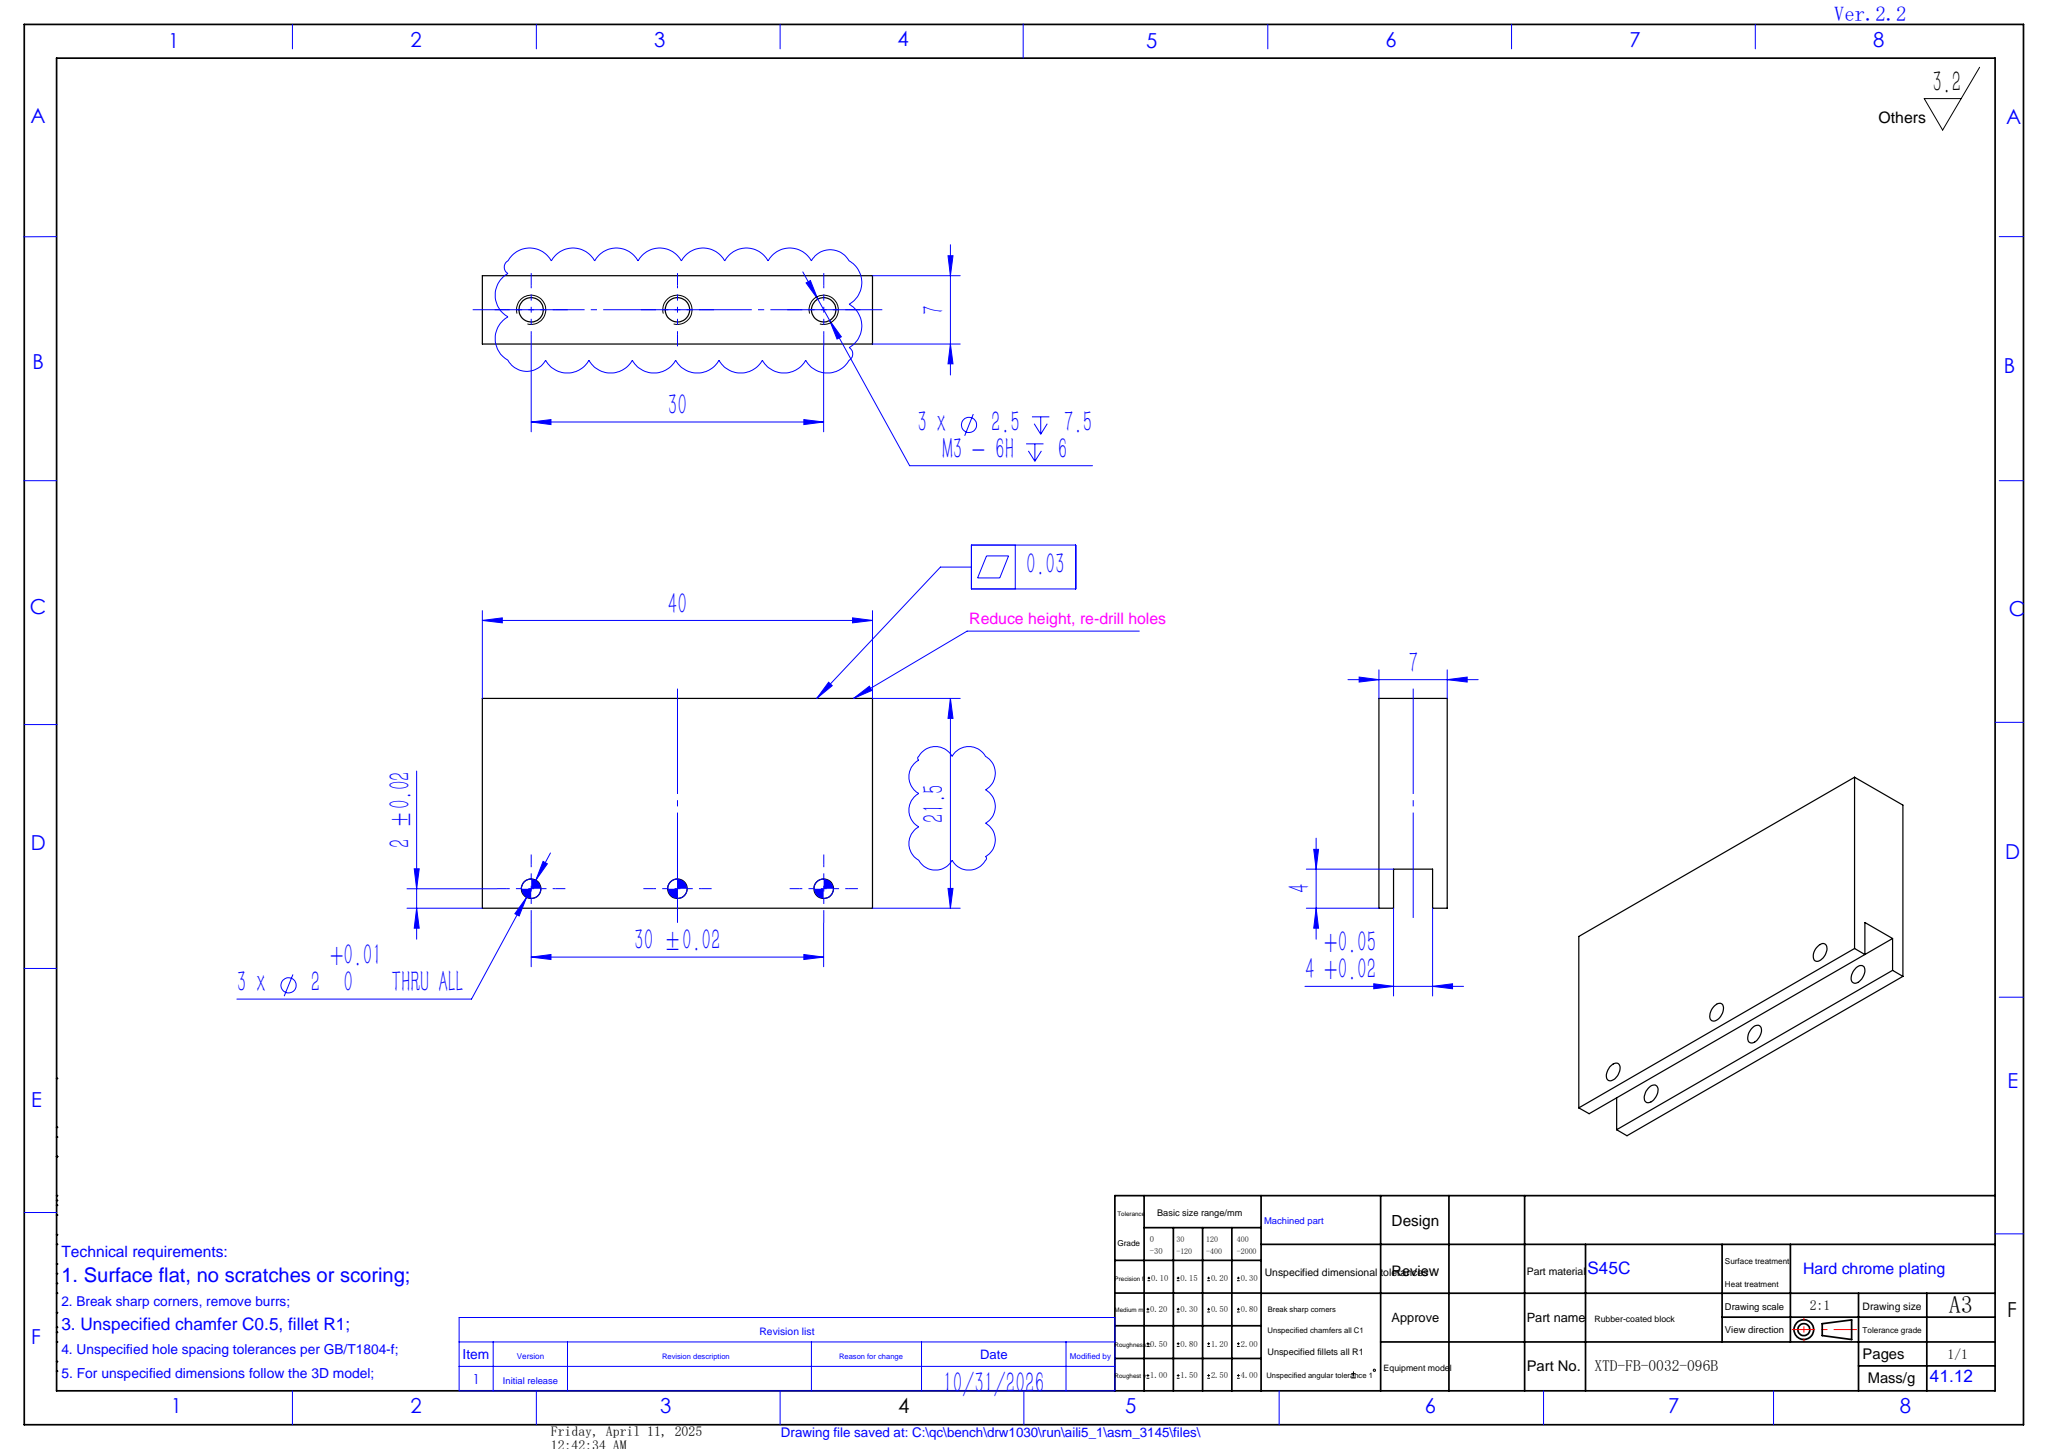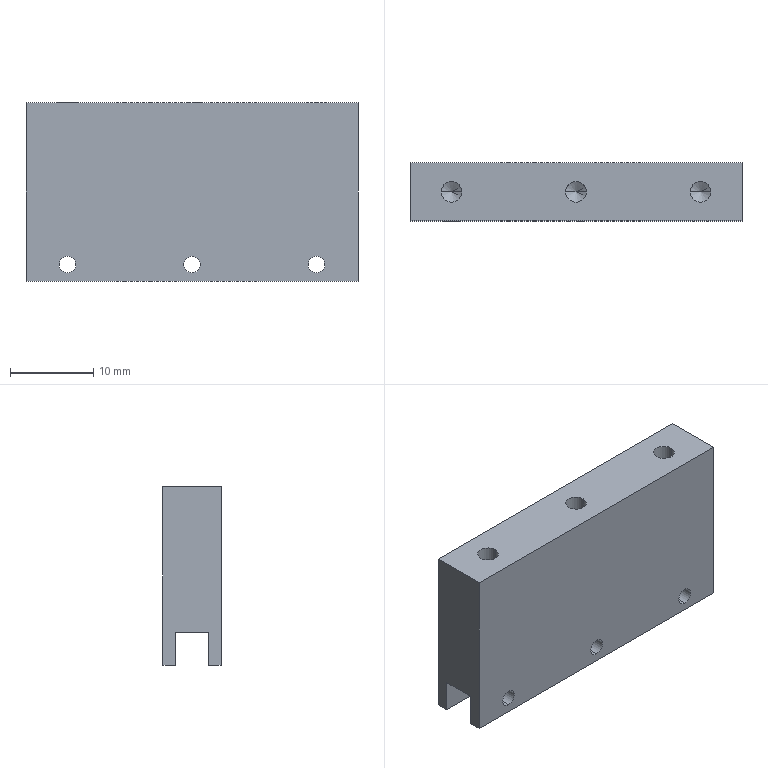Part | SolidWorks | features HoleWzd 2, Cut 1, Extrusion 1 | 1 solid | 34 faces | box 40 x 7 x 21.5 mm | volume 5238 mm3 | cylinder 18 | plane 10 | cone 6 | commonest cylinder face diameters 2 x12 2.5 x6
STEP:
#1=CARTESIAN_POINT('',(-15.,2.,1.));
#2=VERTEX_POINT('',#1);
#3=CARTESIAN_POINT('',(-15.,2.,3.));
#4=VERTEX_POINT('',#3);
#5=CARTESIAN_POINT('',(-15.,2.,2.));
#6=DIRECTION('',(0.,1.,0.));
#7=DIRECTION('',(0.,0.,1.));
#8=AXIS2_PLACEMENT_3D('',#5,#6,#7);
#9=CIRCLE('',#8,1.);
#10=EDGE_CURVE('',#2,#4,#9,.T.);
#11=ORIENTED_EDGE('',*,*,#10,.F.);
#12=CARTESIAN_POINT('',(-15.,3.5,1.));
#13=VERTEX_POINT('',#12);
#14=CARTESIAN_POINT('',(-15.,3.5,1.));
#15=DIRECTION('',(0.,1.,0.));
#16=VECTOR('',#15,1000.);
#17=LINE('',#14,#16);
#18=EDGE_CURVE('',#2,#13,#17,.T.);
#19=ORIENTED_EDGE('',*,*,#18,.T.);
#20=CARTESIAN_POINT('',(-15.,3.5,3.));
#21=VERTEX_POINT('',#20);
#22=CARTESIAN_POINT('',(-15.,3.5,2.));
#23=DIRECTION('',(0.,1.,0.));
#24=DIRECTION('',(0.,0.,1.));
#25=AXIS2_PLACEMENT_3D('',#22,#23,#24);
#26=CIRCLE('',#25,1.);
#27=EDGE_CURVE('',#13,#21,#26,.T.);
#28=ORIENTED_EDGE('',*,*,#27,.T.);
#29=CARTESIAN_POINT('',(-15.,3.5,3.));
#30=DIRECTION('',(0.,1.,0.));
#31=VECTOR('',#30,1000.);
#32=LINE('',#29,#31);
#33=EDGE_CURVE('',#4,#21,#32,.T.);
#34=ORIENTED_EDGE('',*,*,#33,.F.);
#35=EDGE_LOOP('',(#11,#19,#28,#34));
#36=FACE_OUTER_BOUND('',#35,.T.);
#37=CARTESIAN_POINT('',(-15.,3.5,2.));
#38=DIRECTION('',(0.,1.,0.));
#39=DIRECTION('',(0.,0.,1.));
#40=AXIS2_PLACEMENT_3D('',#37,#38,#39);
#41=CYLINDRICAL_SURFACE('',#40,1.);
#42=ADVANCED_FACE('',(#36),#41,.F.);
#43=CARTESIAN_POINT('',(-15.,-3.5,1.));
#44=VERTEX_POINT('',#43);
#45=CARTESIAN_POINT('',(-15.,-3.5,3.));
#46=VERTEX_POINT('',#45);
#47=CARTESIAN_POINT('',(-15.,-3.5,2.));
#48=DIRECTION('',(0.,1.,0.));
#49=DIRECTION('',(0.,0.,1.));
#50=AXIS2_PLACEMENT_3D('',#47,#48,#49);
#51=CIRCLE('',#50,1.);
#52=EDGE_CURVE('',#44,#46,#51,.T.);
#53=ORIENTED_EDGE('',*,*,#52,.F.);
#54=CARTESIAN_POINT('',(-15.,-2.,1.));
#55=VERTEX_POINT('',#54);
#56=CARTESIAN_POINT('',(-15.,3.5,1.));
#57=DIRECTION('',(0.,1.,0.));
#58=VECTOR('',#57,1000.);
#59=LINE('',#56,#58);
#60=EDGE_CURVE('',#44,#55,#59,.T.);
#61=ORIENTED_EDGE('',*,*,#60,.T.);
#62=CARTESIAN_POINT('',(-15.,-2.,3.));
#63=VERTEX_POINT('',#62);
#64=CARTESIAN_POINT('',(-15.,-2.,2.));
#65=DIRECTION('',(0.,-1.,0.));
#66=DIRECTION('',(0.,0.,-1.));
#67=AXIS2_PLACEMENT_3D('',#64,#65,#66);
#68=CIRCLE('',#67,1.);
#69=EDGE_CURVE('',#63,#55,#68,.T.);
#70=ORIENTED_EDGE('',*,*,#69,.F.);
#71=CARTESIAN_POINT('',(-15.,3.5,3.));
#72=DIRECTION('',(0.,1.,0.));
#73=VECTOR('',#72,1000.);
#74=LINE('',#71,#73);
#75=EDGE_CURVE('',#46,#63,#74,.T.);
#76=ORIENTED_EDGE('',*,*,#75,.F.);
#77=EDGE_LOOP('',(#53,#61,#70,#76));
#78=FACE_OUTER_BOUND('',#77,.T.);
#79=CARTESIAN_POINT('',(-15.,3.5,2.));
#80=DIRECTION('',(0.,1.,0.));
#81=DIRECTION('',(0.,0.,1.));
#82=AXIS2_PLACEMENT_3D('',#79,#80,#81);
#83=CYLINDRICAL_SURFACE('',#82,1.);
#84=ADVANCED_FACE('',(#78),#83,.F.);
#85=CARTESIAN_POINT('',(0.,2.,1.));
#86=VERTEX_POINT('',#85);
#87=CARTESIAN_POINT('',(0.,2.,3.));
#88=VERTEX_POINT('',#87);
#89=CARTESIAN_POINT('',(0.,2.,2.));
#90=DIRECTION('',(0.,1.,0.));
#91=DIRECTION('',(0.,0.,1.));
#92=AXIS2_PLACEMENT_3D('',#89,#90,#91);
#93=CIRCLE('',#92,1.);
#94=EDGE_CURVE('',#86,#88,#93,.T.);
#95=ORIENTED_EDGE('',*,*,#94,.F.);
#96=CARTESIAN_POINT('',(0.,3.5,1.));
#97=VERTEX_POINT('',#96);
#98=CARTESIAN_POINT('',(0.,3.5,1.));
#99=DIRECTION('',(0.,1.,0.));
#100=VECTOR('',#99,1000.);
#101=LINE('',#98,#100);
#102=EDGE_CURVE('',#86,#97,#101,.T.);
#103=ORIENTED_EDGE('',*,*,#102,.T.);
#104=CARTESIAN_POINT('',(0.,3.5,3.));
#105=VERTEX_POINT('',#104);
#106=CARTESIAN_POINT('',(0.,3.5,2.));
#107=DIRECTION('',(0.,1.,0.));
#108=DIRECTION('',(0.,0.,1.));
#109=AXIS2_PLACEMENT_3D('',#106,#107,#108);
#110=CIRCLE('',#109,1.);
#111=EDGE_CURVE('',#97,#105,#110,.T.);
#112=ORIENTED_EDGE('',*,*,#111,.T.);
#113=CARTESIAN_POINT('',(0.,3.5,3.));
#114=DIRECTION('',(0.,1.,0.));
#115=VECTOR('',#114,1000.);
#116=LINE('',#113,#115);
#117=EDGE_CURVE('',#88,#105,#116,.T.);
#118=ORIENTED_EDGE('',*,*,#117,.F.);
#119=EDGE_LOOP('',(#95,#103,#112,#118));
#120=FACE_OUTER_BOUND('',#119,.T.);
#121=CARTESIAN_POINT('',(0.,3.5,2.));
#122=DIRECTION('',(0.,1.,0.));
#123=DIRECTION('',(0.,0.,1.));
#124=AXIS2_PLACEMENT_3D('',#121,#122,#123);
#125=CYLINDRICAL_SURFACE('',#124,1.);
#126=ADVANCED_FACE('',(#120),#125,.F.);
#127=CARTESIAN_POINT('',(0.,-3.5,1.));
#128=VERTEX_POINT('',#127);
#129=CARTESIAN_POINT('',(0.,-3.5,3.));
#130=VERTEX_POINT('',#129);
#131=CARTESIAN_POINT('',(0.,-3.5,2.));
#132=DIRECTION('',(0.,1.,0.));
#133=DIRECTION('',(0.,0.,1.));
#134=AXIS2_PLACEMENT_3D('',#131,#132,#133);
#135=CIRCLE('',#134,1.);
#136=EDGE_CURVE('',#128,#130,#135,.T.);
#137=ORIENTED_EDGE('',*,*,#136,.F.);
#138=CARTESIAN_POINT('',(0.,-2.,1.));
#139=VERTEX_POINT('',#138);
#140=CARTESIAN_POINT('',(0.,3.5,1.));
#141=DIRECTION('',(0.,1.,0.));
#142=VECTOR('',#141,1000.);
#143=LINE('',#140,#142);
#144=EDGE_CURVE('',#128,#139,#143,.T.);
#145=ORIENTED_EDGE('',*,*,#144,.T.);
#146=CARTESIAN_POINT('',(0.,-2.,3.));
#147=VERTEX_POINT('',#146);
#148=CARTESIAN_POINT('',(0.,-2.,2.));
#149=DIRECTION('',(0.,-1.,0.));
#150=DIRECTION('',(0.,0.,-1.));
#151=AXIS2_PLACEMENT_3D('',#148,#149,#150);
#152=CIRCLE('',#151,1.);
#153=EDGE_CURVE('',#147,#139,#152,.T.);
#154=ORIENTED_EDGE('',*,*,#153,.F.);
#155=CARTESIAN_POINT('',(0.,3.5,3.));
#156=DIRECTION('',(0.,1.,0.));
#157=VECTOR('',#156,1000.);
#158=LINE('',#155,#157);
#159=EDGE_CURVE('',#130,#147,#158,.T.);
#160=ORIENTED_EDGE('',*,*,#159,.F.);
#161=EDGE_LOOP('',(#137,#145,#154,#160));
#162=FACE_OUTER_BOUND('',#161,.T.);
#163=CARTESIAN_POINT('',(0.,3.5,2.));
#164=DIRECTION('',(0.,1.,0.));
#165=DIRECTION('',(0.,0.,1.));
#166=AXIS2_PLACEMENT_3D('',#163,#164,#165);
#167=CYLINDRICAL_SURFACE('',#166,1.);
#168=ADVANCED_FACE('',(#162),#167,.F.);
#169=CARTESIAN_POINT('',(15.,2.,1.));
#170=VERTEX_POINT('',#169);
#171=CARTESIAN_POINT('',(15.,2.,3.));
#172=VERTEX_POINT('',#171);
#173=CARTESIAN_POINT('',(15.,2.,2.));
#174=DIRECTION('',(0.,1.,0.));
#175=DIRECTION('',(0.,0.,1.));
#176=AXIS2_PLACEMENT_3D('',#173,#174,#175);
#177=CIRCLE('',#176,1.);
#178=EDGE_CURVE('',#170,#172,#177,.T.);
#179=ORIENTED_EDGE('',*,*,#178,.F.);
#180=CARTESIAN_POINT('',(15.,3.5,1.));
#181=VERTEX_POINT('',#180);
#182=CARTESIAN_POINT('',(15.,3.5,1.));
#183=DIRECTION('',(0.,1.,0.));
#184=VECTOR('',#183,1000.);
#185=LINE('',#182,#184);
#186=EDGE_CURVE('',#170,#181,#185,.T.);
#187=ORIENTED_EDGE('',*,*,#186,.T.);
#188=CARTESIAN_POINT('',(15.,3.5,3.));
#189=VERTEX_POINT('',#188);
#190=CARTESIAN_POINT('',(15.,3.5,2.));
#191=DIRECTION('',(0.,1.,0.));
#192=DIRECTION('',(0.,0.,1.));
#193=AXIS2_PLACEMENT_3D('',#190,#191,#192);
#194=CIRCLE('',#193,1.);
#195=EDGE_CURVE('',#181,#189,#194,.T.);
#196=ORIENTED_EDGE('',*,*,#195,.T.);
#197=CARTESIAN_POINT('',(15.,3.5,3.));
#198=DIRECTION('',(0.,1.,0.));
#199=VECTOR('',#198,1000.);
#200=LINE('',#197,#199);
#201=EDGE_CURVE('',#172,#189,#200,.T.);
#202=ORIENTED_EDGE('',*,*,#201,.F.);
#203=EDGE_LOOP('',(#179,#187,#196,#202));
#204=FACE_OUTER_BOUND('',#203,.T.);
#205=CARTESIAN_POINT('',(15.,3.5,2.));
#206=DIRECTION('',(0.,1.,0.));
#207=DIRECTION('',(0.,0.,1.));
#208=AXIS2_PLACEMENT_3D('',#205,#206,#207);
#209=CYLINDRICAL_SURFACE('',#208,1.);
#210=ADVANCED_FACE('',(#204),#209,.F.);
#211=CARTESIAN_POINT('',(15.,-3.5,1.));
#212=VERTEX_POINT('',#211);
#213=CARTESIAN_POINT('',(15.,-3.5,3.));
#214=VERTEX_POINT('',#213);
#215=CARTESIAN_POINT('',(15.,-3.5,2.));
#216=DIRECTION('',(0.,1.,0.));
#217=DIRECTION('',(0.,0.,1.));
#218=AXIS2_PLACEMENT_3D('',#215,#216,#217);
#219=CIRCLE('',#218,1.);
#220=EDGE_CURVE('',#212,#214,#219,.T.);
#221=ORIENTED_EDGE('',*,*,#220,.F.);
#222=CARTESIAN_POINT('',(15.,-2.,1.));
#223=VERTEX_POINT('',#222);
#224=CARTESIAN_POINT('',(15.,3.5,1.));
#225=DIRECTION('',(0.,1.,0.));
#226=VECTOR('',#225,1000.);
#227=LINE('',#224,#226);
#228=EDGE_CURVE('',#212,#223,#227,.T.);
#229=ORIENTED_EDGE('',*,*,#228,.T.);
#230=CARTESIAN_POINT('',(15.,-2.,3.));
#231=VERTEX_POINT('',#230);
#232=CARTESIAN_POINT('',(15.,-2.,2.));
#233=DIRECTION('',(0.,-1.,0.));
#234=DIRECTION('',(0.,0.,-1.));
#235=AXIS2_PLACEMENT_3D('',#232,#233,#234);
#236=CIRCLE('',#235,1.);
#237=EDGE_CURVE('',#231,#223,#236,.T.);
#238=ORIENTED_EDGE('',*,*,#237,.F.);
#239=CARTESIAN_POINT('',(15.,3.5,3.));
#240=DIRECTION('',(0.,1.,0.));
#241=VECTOR('',#240,1000.);
#242=LINE('',#239,#241);
#243=EDGE_CURVE('',#214,#231,#242,.T.);
#244=ORIENTED_EDGE('',*,*,#243,.F.);
#245=EDGE_LOOP('',(#221,#229,#238,#244));
#246=FACE_OUTER_BOUND('',#245,.T.);
#247=CARTESIAN_POINT('',(15.,3.5,2.));
#248=DIRECTION('',(0.,1.,0.));
#249=DIRECTION('',(0.,0.,1.));
#250=AXIS2_PLACEMENT_3D('',#247,#248,#249);
#251=CYLINDRICAL_SURFACE('',#250,1.);
#252=ADVANCED_FACE('',(#246),#251,.F.);
#253=CARTESIAN_POINT('',(-16.25,0.,14.));
#254=VERTEX_POINT('',#253);
#255=CARTESIAN_POINT('',(-13.75,0.,14.));
#256=VERTEX_POINT('',#255);
#257=CARTESIAN_POINT('',(-15.,0.,14.));
#258=DIRECTION('',(0.,0.,1.));
#259=DIRECTION('',(1.,0.,0.));
#260=AXIS2_PLACEMENT_3D('',#257,#258,#259);
#261=CIRCLE('',#260,1.25);
#262=EDGE_CURVE('',#254,#256,#261,.T.);
#263=ORIENTED_EDGE('',*,*,#262,.F.);
#264=CARTESIAN_POINT('',(-16.25,0.,21.5));
#265=VERTEX_POINT('',#264);
#266=CARTESIAN_POINT('',(-16.25,0.,21.5));
#267=DIRECTION('',(0.,0.,1.));
#268=VECTOR('',#267,1000.);
#269=LINE('',#266,#268);
#270=EDGE_CURVE('',#254,#265,#269,.T.);
#271=ORIENTED_EDGE('',*,*,#270,.T.);
#272=CARTESIAN_POINT('',(-13.75,0.,21.5));
#273=VERTEX_POINT('',#272);
#274=CARTESIAN_POINT('',(-15.,0.,21.5));
#275=DIRECTION('',(0.,0.,1.));
#276=DIRECTION('',(1.,0.,0.));
#277=AXIS2_PLACEMENT_3D('',#274,#275,#276);
#278=CIRCLE('',#277,1.25);
#279=EDGE_CURVE('',#265,#273,#278,.T.);
#280=ORIENTED_EDGE('',*,*,#279,.T.);
#281=CARTESIAN_POINT('',(-13.75,0.,21.5));
#282=DIRECTION('',(0.,0.,1.));
#283=VECTOR('',#282,1000.);
#284=LINE('',#281,#283);
#285=EDGE_CURVE('',#256,#273,#284,.T.);
#286=ORIENTED_EDGE('',*,*,#285,.F.);
#287=EDGE_LOOP('',(#263,#271,#280,#286));
#288=FACE_OUTER_BOUND('',#287,.T.);
#289=CARTESIAN_POINT('',(-15.,0.,21.5));
#290=DIRECTION('',(0.,0.,1.));
#291=DIRECTION('',(1.,0.,0.));
#292=AXIS2_PLACEMENT_3D('',#289,#290,#291);
#293=CYLINDRICAL_SURFACE('',#292,1.25);
#294=ADVANCED_FACE('',(#288),#293,.F.);
#295=CARTESIAN_POINT('',(-15.,0.,13.249));
#296=VERTEX_POINT('',#295);
#297=CARTESIAN_POINT('',(-13.75,0.,14.));
#298=DIRECTION('',(0.8572,0.,0.515));
#299=VECTOR('',#298,1000.);
#300=LINE('',#297,#299);
#301=EDGE_CURVE('',#296,#256,#300,.T.);
#302=ORIENTED_EDGE('',*,*,#301,.F.);
#303=CARTESIAN_POINT('',(-16.25,0.,14.));
#304=DIRECTION('',(-0.8572,0.,0.515));
#305=VECTOR('',#304,1000.);
#306=LINE('',#303,#305);
#307=EDGE_CURVE('',#296,#254,#306,.T.);
#308=ORIENTED_EDGE('',*,*,#307,.T.);
#309=ORIENTED_EDGE('',*,*,#262,.T.);
#310=EDGE_LOOP('',(#302,#308,#309));
#311=FACE_OUTER_BOUND('',#310,.T.);
#312=CARTESIAN_POINT('',(-15.,0.,14.));
#313=DIRECTION('',(0.,0.,1.));
#314=DIRECTION('',(1.,0.,0.));
#315=AXIS2_PLACEMENT_3D('',#312,#313,#314);
#316=CONICAL_SURFACE('',#315,1.25,1.03);
#317=ADVANCED_FACE('',(#311),#316,.F.);
#318=CARTESIAN_POINT('',(-1.25,0.,14.));
#319=VERTEX_POINT('',#318);
#320=CARTESIAN_POINT('',(1.25,0.,14.));
#321=VERTEX_POINT('',#320);
#322=CARTESIAN_POINT('',(0.,0.,14.));
#323=DIRECTION('',(0.,0.,1.));
#324=DIRECTION('',(1.,0.,0.));
#325=AXIS2_PLACEMENT_3D('',#322,#323,#324);
#326=CIRCLE('',#325,1.25);
#327=EDGE_CURVE('',#319,#321,#326,.T.);
#328=ORIENTED_EDGE('',*,*,#327,.F.);
#329=CARTESIAN_POINT('',(-1.25,0.,21.5));
#330=VERTEX_POINT('',#329);
#331=CARTESIAN_POINT('',(-1.25,0.,21.5));
#332=DIRECTION('',(0.,0.,1.));
#333=VECTOR('',#332,1000.);
#334=LINE('',#331,#333);
#335=EDGE_CURVE('',#319,#330,#334,.T.);
#336=ORIENTED_EDGE('',*,*,#335,.T.);
#337=CARTESIAN_POINT('',(1.25,0.,21.5));
#338=VERTEX_POINT('',#337);
#339=CARTESIAN_POINT('',(0.,0.,21.5));
#340=DIRECTION('',(0.,0.,1.));
#341=DIRECTION('',(1.,0.,0.));
#342=AXIS2_PLACEMENT_3D('',#339,#340,#341);
#343=CIRCLE('',#342,1.25);
#344=EDGE_CURVE('',#330,#338,#343,.T.);
#345=ORIENTED_EDGE('',*,*,#344,.T.);
#346=CARTESIAN_POINT('',(1.25,0.,21.5));
#347=DIRECTION('',(0.,0.,1.));
#348=VECTOR('',#347,1000.);
#349=LINE('',#346,#348);
#350=EDGE_CURVE('',#321,#338,#349,.T.);
#351=ORIENTED_EDGE('',*,*,#350,.F.);
#352=EDGE_LOOP('',(#328,#336,#345,#351));
#353=FACE_OUTER_BOUND('',#352,.T.);
#354=CARTESIAN_POINT('',(0.,0.,21.5));
#355=DIRECTION('',(0.,0.,1.));
#356=DIRECTION('',(1.,0.,0.));
#357=AXIS2_PLACEMENT_3D('',#354,#355,#356);
#358=CYLINDRICAL_SURFACE('',#357,1.25);
#359=ADVANCED_FACE('',(#353),#358,.F.);
#360=CARTESIAN_POINT('',(0.,0.,13.249));
#361=VERTEX_POINT('',#360);
#362=CARTESIAN_POINT('',(1.25,0.,14.));
#363=DIRECTION('',(0.8572,0.,0.515));
#364=VECTOR('',#363,1000.);
#365=LINE('',#362,#364);
#366=EDGE_CURVE('',#361,#321,#365,.T.);
#367=ORIENTED_EDGE('',*,*,#366,.F.);
#368=CARTESIAN_POINT('',(-1.25,0.,14.));
#369=DIRECTION('',(-0.8572,0.,0.515));
#370=VECTOR('',#369,1000.);
#371=LINE('',#368,#370);
#372=EDGE_CURVE('',#361,#319,#371,.T.);
#373=ORIENTED_EDGE('',*,*,#372,.T.);
#374=ORIENTED_EDGE('',*,*,#327,.T.);
#375=EDGE_LOOP('',(#367,#373,#374));
#376=FACE_OUTER_BOUND('',#375,.T.);
#377=CARTESIAN_POINT('',(0.,0.,14.));
#378=DIRECTION('',(0.,0.,1.));
#379=DIRECTION('',(1.,0.,0.));
#380=AXIS2_PLACEMENT_3D('',#377,#378,#379);
#381=CONICAL_SURFACE('',#380,1.25,1.03);
#382=ADVANCED_FACE('',(#376),#381,.F.);
#383=CARTESIAN_POINT('',(13.75,0.,14.));
#384=VERTEX_POINT('',#383);
#385=CARTESIAN_POINT('',(16.25,0.,14.));
#386=VERTEX_POINT('',#385);
#387=CARTESIAN_POINT('',(15.,0.,14.));
#388=DIRECTION('',(0.,0.,1.));
#389=DIRECTION('',(1.,0.,0.));
#390=AXIS2_PLACEMENT_3D('',#387,#388,#389);
#391=CIRCLE('',#390,1.25);
#392=EDGE_CURVE('',#384,#386,#391,.T.);
#393=ORIENTED_EDGE('',*,*,#392,.F.);
#394=CARTESIAN_POINT('',(13.75,0.,21.5));
#395=VERTEX_POINT('',#394);
#396=CARTESIAN_POINT('',(13.75,0.,21.5));
#397=DIRECTION('',(0.,0.,1.));
#398=VECTOR('',#397,1000.);
#399=LINE('',#396,#398);
#400=EDGE_CURVE('',#384,#395,#399,.T.);
#401=ORIENTED_EDGE('',*,*,#400,.T.);
#402=CARTESIAN_POINT('',(16.25,0.,21.5));
#403=VERTEX_POINT('',#402);
#404=CARTESIAN_POINT('',(15.,0.,21.5));
#405=DIRECTION('',(0.,0.,1.));
#406=DIRECTION('',(1.,0.,0.));
#407=AXIS2_PLACEMENT_3D('',#404,#405,#406);
#408=CIRCLE('',#407,1.25);
#409=EDGE_CURVE('',#395,#403,#408,.T.);
#410=ORIENTED_EDGE('',*,*,#409,.T.);
#411=CARTESIAN_POINT('',(16.25,0.,21.5));
#412=DIRECTION('',(0.,0.,1.));
#413=VECTOR('',#412,1000.);
#414=LINE('',#411,#413);
#415=EDGE_CURVE('',#386,#403,#414,.T.);
#416=ORIENTED_EDGE('',*,*,#415,.F.);
#417=EDGE_LOOP('',(#393,#401,#410,#416));
#418=FACE_OUTER_BOUND('',#417,.T.);
#419=CARTESIAN_POINT('',(15.,0.,21.5));
#420=DIRECTION('',(0.,0.,1.));
#421=DIRECTION('',(1.,0.,0.));
#422=AXIS2_PLACEMENT_3D('',#419,#420,#421);
#423=CYLINDRICAL_SURFACE('',#422,1.25);
#424=ADVANCED_FACE('',(#418),#423,.F.);
#425=CARTESIAN_POINT('',(15.,0.,13.249));
#426=VERTEX_POINT('',#425);
#427=CARTESIAN_POINT('',(16.25,0.,14.));
#428=DIRECTION('',(0.8572,0.,0.515));
#429=VECTOR('',#428,1000.);
#430=LINE('',#427,#429);
#431=EDGE_CURVE('',#426,#386,#430,.T.);
#432=ORIENTED_EDGE('',*,*,#431,.F.);
#433=CARTESIAN_POINT('',(13.75,0.,14.));
#434=DIRECTION('',(-0.8572,0.,0.515));
#435=VECTOR('',#434,1000.);
#436=LINE('',#433,#435);
#437=EDGE_CURVE('',#426,#384,#436,.T.);
#438=ORIENTED_EDGE('',*,*,#437,.T.);
#439=ORIENTED_EDGE('',*,*,#392,.T.);
#440=EDGE_LOOP('',(#432,#438,#439));
#441=FACE_OUTER_BOUND('',#440,.T.);
#442=CARTESIAN_POINT('',(15.,0.,14.));
#443=DIRECTION('',(0.,0.,1.));
#444=DIRECTION('',(1.,0.,0.));
#445=AXIS2_PLACEMENT_3D('',#442,#443,#444);
#446=CONICAL_SURFACE('',#445,1.25,1.03);
#447=ADVANCED_FACE('',(#441),#446,.F.);
#448=CARTESIAN_POINT('',(20.,2.,0.));
#449=VERTEX_POINT('',#448);
#450=CARTESIAN_POINT('',(20.,3.5,0.));
#451=VERTEX_POINT('',#450);
#452=CARTESIAN_POINT('',(20.,3.5,0.));
#453=DIRECTION('',(0.,1.,0.));
#454=VECTOR('',#453,1000.);
#455=LINE('',#452,#454);
#456=EDGE_CURVE('',#449,#451,#455,.T.);
#457=ORIENTED_EDGE('',*,*,#456,.F.);
#458=CARTESIAN_POINT('',(-20.,2.,0.));
#459=VERTEX_POINT('',#458);
#460=CARTESIAN_POINT('',(-20.,2.,0.));
#461=DIRECTION('',(1.,0.,0.));
#462=VECTOR('',#461,1000.);
#463=LINE('',#460,#462);
#464=EDGE_CURVE('',#459,#449,#463,.T.);
#465=ORIENTED_EDGE('',*,*,#464,.F.);
#466=CARTESIAN_POINT('',(-20.,3.5,0.));
#467=VERTEX_POINT('',#466);
#468=CARTESIAN_POINT('',(-20.,3.5,0.));
#469=DIRECTION('',(0.,-1.,0.));
#470=VECTOR('',#469,1000.);
#471=LINE('',#468,#470);
#472=EDGE_CURVE('',#467,#459,#471,.T.);
#473=ORIENTED_EDGE('',*,*,#472,.F.);
#474=CARTESIAN_POINT('',(-20.,3.5,0.));
#475=DIRECTION('',(-1.,0.,0.));
#476=VECTOR('',#475,1000.);
#477=LINE('',#474,#476);
#478=EDGE_CURVE('',#451,#467,#477,.T.);
#479=ORIENTED_EDGE('',*,*,#478,.F.);
#480=EDGE_LOOP('',(#457,#465,#473,#479));
#481=FACE_OUTER_BOUND('',#480,.T.);
#482=CARTESIAN_POINT('',(0.,0.,0.));
#483=DIRECTION('',(0.,0.,1.));
#484=DIRECTION('',(1.,0.,0.));
#485=AXIS2_PLACEMENT_3D('',#482,#483,#484);
#486=PLANE('',#485);
#487=ADVANCED_FACE('',(#481),#486,.F.);
#488=CARTESIAN_POINT('',(20.,2.,4.));
#489=VERTEX_POINT('',#488);
#490=CARTESIAN_POINT('',(20.,-2.,4.));
#491=VERTEX_POINT('',#490);
#492=CARTESIAN_POINT('',(20.,2.,4.));
#493=DIRECTION('',(0.,-1.,0.));
#494=VECTOR('',#493,1000.);
#495=LINE('',#492,#494);
#496=EDGE_CURVE('',#489,#491,#495,.T.);
#497=ORIENTED_EDGE('',*,*,#496,.F.);
#498=CARTESIAN_POINT('',(20.,2.,4.));
#499=DIRECTION('',(0.,0.,1.));
#500=VECTOR('',#499,1000.);
#501=LINE('',#498,#500);
#502=EDGE_CURVE('',#449,#489,#501,.T.);
#503=ORIENTED_EDGE('',*,*,#502,.F.);
#504=ORIENTED_EDGE('',*,*,#456,.T.);
#505=CARTESIAN_POINT('',(20.,3.5,21.5));
#506=VERTEX_POINT('',#505);
#507=CARTESIAN_POINT('',(20.,3.5,21.5));
#508=DIRECTION('',(0.,0.,-1.));
#509=VECTOR('',#508,1000.);
#510=LINE('',#507,#509);
#511=EDGE_CURVE('',#506,#451,#510,.T.);
#512=ORIENTED_EDGE('',*,*,#511,.F.);
#513=CARTESIAN_POINT('',(20.,-3.5,21.5));
#514=VERTEX_POINT('',#513);
#515=CARTESIAN_POINT('',(20.,3.5,21.5));
#516=DIRECTION('',(0.,1.,0.));
#517=VECTOR('',#516,1000.);
#518=LINE('',#515,#517);
#519=EDGE_CURVE('',#514,#506,#518,.T.);
#520=ORIENTED_EDGE('',*,*,#519,.F.);
#521=CARTESIAN_POINT('',(20.,-3.5,0.));
#522=VERTEX_POINT('',#521);
#523=CARTESIAN_POINT('',(20.,-3.5,21.5));
#524=DIRECTION('',(0.,0.,-1.));
#525=VECTOR('',#524,1000.);
#526=LINE('',#523,#525);
#527=EDGE_CURVE('',#514,#522,#526,.T.);
#528=ORIENTED_EDGE('',*,*,#527,.T.);
#529=CARTESIAN_POINT('',(20.,-2.,0.));
#530=VERTEX_POINT('',#529);
#531=CARTESIAN_POINT('',(20.,3.5,0.));
#532=DIRECTION('',(0.,1.,0.));
#533=VECTOR('',#532,1000.);
#534=LINE('',#531,#533);
#535=EDGE_CURVE('',#522,#530,#534,.T.);
#536=ORIENTED_EDGE('',*,*,#535,.T.);
#537=CARTESIAN_POINT('',(20.,-2.,4.));
#538=DIRECTION('',(0.,0.,-1.));
#539=VECTOR('',#538,1000.);
#540=LINE('',#537,#539);
#541=EDGE_CURVE('',#491,#530,#540,.T.);
#542=ORIENTED_EDGE('',*,*,#541,.F.);
#543=EDGE_LOOP('',(#497,#503,#504,#512,#520,#528,#536,#542));
#544=FACE_OUTER_BOUND('',#543,.T.);
#545=CARTESIAN_POINT('',(20.,3.5,21.5));
#546=DIRECTION('',(-1.,0.,0.));
#547=DIRECTION('',(0.,0.,1.));
#548=AXIS2_PLACEMENT_3D('',#545,#546,#547);
#549=PLANE('',#548);
#550=ADVANCED_FACE('',(#544),#549,.F.);
#551=CARTESIAN_POINT('',(-15.,3.5,2.));
#552=DIRECTION('',(0.,1.,0.));
#553=DIRECTION('',(0.,0.,1.));
#554=AXIS2_PLACEMENT_3D('',#551,#552,#553);
#555=CIRCLE('',#554,1.);
#556=EDGE_CURVE('',#21,#13,#555,.T.);
#557=ORIENTED_EDGE('',*,*,#556,.F.);
#558=ORIENTED_EDGE('',*,*,#27,.F.);
#559=EDGE_LOOP('',(#557,#558));
#560=FACE_BOUND('',#559,.T.);
#561=CARTESIAN_POINT('',(0.,3.5,2.));
#562=DIRECTION('',(0.,1.,0.));
#563=DIRECTION('',(0.,0.,1.));
#564=AXIS2_PLACEMENT_3D('',#561,#562,#563);
#565=CIRCLE('',#564,1.);
#566=EDGE_CURVE('',#105,#97,#565,.T.);
#567=ORIENTED_EDGE('',*,*,#566,.F.);
#568=ORIENTED_EDGE('',*,*,#111,.F.);
#569=EDGE_LOOP('',(#567,#568));
#570=FACE_BOUND('',#569,.T.);
#571=CARTESIAN_POINT('',(15.,3.5,2.));
#572=DIRECTION('',(0.,1.,0.));
#573=DIRECTION('',(0.,0.,1.));
#574=AXIS2_PLACEMENT_3D('',#571,#572,#573);
#575=CIRCLE('',#574,1.);
#576=EDGE_CURVE('',#189,#181,#575,.T.);
#577=ORIENTED_EDGE('',*,*,#576,.F.);
#578=ORIENTED_EDGE('',*,*,#195,.F.);
#579=EDGE_LOOP('',(#577,#578));
#580=FACE_BOUND('',#579,.T.);
#581=ORIENTED_EDGE('',*,*,#478,.T.);
#582=CARTESIAN_POINT('',(-20.,3.5,21.5));
#583=VERTEX_POINT('',#582);
#584=CARTESIAN_POINT('',(-20.,3.5,21.5));
#585=DIRECTION('',(0.,0.,-1.));
#586=VECTOR('',#585,1000.);
#587=LINE('',#584,#586);
#588=EDGE_CURVE('',#583,#467,#587,.T.);
#589=ORIENTED_EDGE('',*,*,#588,.F.);
#590=CARTESIAN_POINT('',(-20.,3.5,21.5));
#591=DIRECTION('',(-1.,0.,0.));
#592=VECTOR('',#591,1000.);
#593=LINE('',#590,#592);
#594=EDGE_CURVE('',#506,#583,#593,.T.);
#595=ORIENTED_EDGE('',*,*,#594,.F.);
#596=ORIENTED_EDGE('',*,*,#511,.T.);
#597=EDGE_LOOP('',(#581,#589,#595,#596));
#598=FACE_OUTER_BOUND('',#597,.T.);
#599=CARTESIAN_POINT('',(-20.,3.5,21.5));
#600=DIRECTION('',(0.,-1.,0.));
#601=DIRECTION('',(0.,0.,-1.));
#602=AXIS2_PLACEMENT_3D('',#599,#600,#601);
#603=PLANE('',#602);
#604=ADVANCED_FACE('',(#560,#570,#580,#598),#603,.F.);
#605=ORIENTED_EDGE('',*,*,#472,.T.);
#606=CARTESIAN_POINT('',(-20.,2.,4.));
#607=VERTEX_POINT('',#606);
#608=CARTESIAN_POINT('',(-20.,2.,4.));
#609=DIRECTION('',(0.,0.,1.));
#610=VECTOR('',#609,1000.);
#611=LINE('',#608,#610);
#612=EDGE_CURVE('',#459,#607,#611,.T.);
#613=ORIENTED_EDGE('',*,*,#612,.T.);
#614=CARTESIAN_POINT('',(-20.,-2.,4.));
#615=VERTEX_POINT('',#614);
#616=CARTESIAN_POINT('',(-20.,2.,4.));
#617=DIRECTION('',(0.,-1.,0.));
#618=VECTOR('',#617,1000.);
#619=LINE('',#616,#618);
#620=EDGE_CURVE('',#607,#615,#619,.T.);
#621=ORIENTED_EDGE('',*,*,#620,.T.);
#622=CARTESIAN_POINT('',(-20.,-2.,0.));
#623=VERTEX_POINT('',#622);
#624=CARTESIAN_POINT('',(-20.,-2.,4.));
#625=DIRECTION('',(0.,0.,-1.));
#626=VECTOR('',#625,1000.);
#627=LINE('',#624,#626);
#628=EDGE_CURVE('',#615,#623,#627,.T.);
#629=ORIENTED_EDGE('',*,*,#628,.T.);
#630=CARTESIAN_POINT('',(-20.,-3.5,0.));
#631=VERTEX_POINT('',#630);
#632=CARTESIAN_POINT('',(-20.,3.5,0.));
#633=DIRECTION('',(0.,-1.,0.));
#634=VECTOR('',#633,1000.);
#635=LINE('',#632,#634);
#636=EDGE_CURVE('',#623,#631,#635,.T.);
#637=ORIENTED_EDGE('',*,*,#636,.T.);
#638=CARTESIAN_POINT('',(-20.,-3.5,21.5));
#639=VERTEX_POINT('',#638);
#640=CARTESIAN_POINT('',(-20.,-3.5,21.5));
#641=DIRECTION('',(0.,0.,-1.));
#642=VECTOR('',#641,1000.);
#643=LINE('',#640,#642);
#644=EDGE_CURVE('',#639,#631,#643,.T.);
#645=ORIENTED_EDGE('',*,*,#644,.F.);
#646=CARTESIAN_POINT('',(-20.,3.5,21.5));
#647=DIRECTION('',(0.,-1.,0.));
#648=VECTOR('',#647,1000.);
#649=LINE('',#646,#648);
#650=EDGE_CURVE('',#583,#639,#649,.T.);
#651=ORIENTED_EDGE('',*,*,#650,.F.);
#652=ORIENTED_EDGE('',*,*,#588,.T.);
#653=EDGE_LOOP('',(#605,#613,#621,#629,#637,#645,#651,#652));
#654=FACE_OUTER_BOUND('',#653,.T.);
#655=CARTESIAN_POINT('',(-20.,3.5,21.5));
#656=DIRECTION('',(1.,0.,0.));
#657=DIRECTION('',(0.,0.,-1.));
#658=AXIS2_PLACEMENT_3D('',#655,#656,#657);
#659=PLANE('',#658);
#660=ADVANCED_FACE('',(#654),#659,.F.);
#661=CARTESIAN_POINT('',(-15.,-3.5,2.));
#662=DIRECTION('',(0.,1.,0.));
#663=DIRECTION('',(0.,0.,1.));
#664=AXIS2_PLACEMENT_3D('',#661,#662,#663);
#665=CIRCLE('',#664,1.);
#666=EDGE_CURVE('',#46,#44,#665,.T.);
#667=ORIENTED_EDGE('',*,*,#666,.T.);
#668=ORIENTED_EDGE('',*,*,#52,.T.);
#669=EDGE_LOOP('',(#667,#668));
#670=FACE_BOUND('',#669,.T.);
#671=CARTESIAN_POINT('',(0.,-3.5,2.));
#672=DIRECTION('',(0.,1.,0.));
#673=DIRECTION('',(0.,0.,1.));
#674=AXIS2_PLACEMENT_3D('',#671,#672,#673);
#675=CIRCLE('',#674,1.);
#676=EDGE_CURVE('',#130,#128,#675,.T.);
#677=ORIENTED_EDGE('',*,*,#676,.T.);
#678=ORIENTED_EDGE('',*,*,#136,.T.);
#679=EDGE_LOOP('',(#677,#678));
#680=FACE_BOUND('',#679,.T.);
#681=CARTESIAN_POINT('',(15.,-3.5,2.));
#682=DIRECTION('',(0.,1.,0.));
#683=DIRECTION('',(0.,0.,1.));
#684=AXIS2_PLACEMENT_3D('',#681,#682,#683);
#685=CIRCLE('',#684,1.);
#686=EDGE_CURVE('',#214,#212,#685,.T.);
#687=ORIENTED_EDGE('',*,*,#686,.T.);
#688=ORIENTED_EDGE('',*,*,#220,.T.);
#689=EDGE_LOOP('',(#687,#688));
#690=FACE_BOUND('',#689,.T.);
#691=CARTESIAN_POINT('',(-20.,-3.5,0.));
#692=DIRECTION('',(1.,0.,0.));
#693=VECTOR('',#692,1000.);
#694=LINE('',#691,#693);
#695=EDGE_CURVE('',#631,#522,#694,.T.);
#696=ORIENTED_EDGE('',*,*,#695,.T.);
#697=ORIENTED_EDGE('',*,*,#527,.F.);
#698=CARTESIAN_POINT('',(-20.,-3.5,21.5));
#699=DIRECTION('',(1.,0.,0.));
#700=VECTOR('',#699,1000.);
#701=LINE('',#698,#700);
#702=EDGE_CURVE('',#639,#514,#701,.T.);
#703=ORIENTED_EDGE('',*,*,#702,.F.);
#704=ORIENTED_EDGE('',*,*,#644,.T.);
#705=EDGE_LOOP('',(#696,#697,#703,#704));
#706=FACE_OUTER_BOUND('',#705,.T.);
#707=CARTESIAN_POINT('',(-20.,-3.5,21.5));
#708=DIRECTION('',(0.,1.,0.));
#709=DIRECTION('',(0.,0.,1.));
#710=AXIS2_PLACEMENT_3D('',#707,#708,#709);
#711=PLANE('',#710);
#712=ADVANCED_FACE('',(#670,#680,#690,#706),#711,.F.);
#713=CARTESIAN_POINT('',(-15.,0.,21.5));
#714=DIRECTION('',(0.,0.,1.));
#715=DIRECTION('',(1.,0.,0.));
#716=AXIS2_PLACEMENT_3D('',#713,#714,#715);
#717=CIRCLE('',#716,1.25);
#718=EDGE_CURVE('',#273,#265,#717,.T.);
#719=ORIENTED_EDGE('',*,*,#718,.F.);
#720=ORIENTED_EDGE('',*,*,#279,.F.);
#721=EDGE_LOOP('',(#719,#720));
#722=FACE_BOUND('',#721,.T.);
#723=CARTESIAN_POINT('',(0.,0.,21.5));
#724=DIRECTION('',(0.,0.,1.));
#725=DIRECTION('',(1.,0.,0.));
#726=AXIS2_PLACEMENT_3D('',#723,#724,#725);
#727=CIRCLE('',#726,1.25);
#728=EDGE_CURVE('',#338,#330,#727,.T.);
#729=ORIENTED_EDGE('',*,*,#728,.F.);
#730=ORIENTED_EDGE('',*,*,#344,.F.);
#731=EDGE_LOOP('',(#729,#730));
#732=FACE_BOUND('',#731,.T.);
#733=CARTESIAN_POINT('',(15.,0.,21.5));
#734=DIRECTION('',(0.,0.,1.));
#735=DIRECTION('',(1.,0.,0.));
#736=AXIS2_PLACEMENT_3D('',#733,#734,#735);
#737=CIRCLE('',#736,1.25);
#738=EDGE_CURVE('',#403,#395,#737,.T.);
#739=ORIENTED_EDGE('',*,*,#738,.F.);
#740=ORIENTED_EDGE('',*,*,#409,.F.);
#741=EDGE_LOOP('',(#739,#740));
#742=FACE_BOUND('',#741,.T.);
#743=ORIENTED_EDGE('',*,*,#519,.T.);
#744=ORIENTED_EDGE('',*,*,#594,.T.);
#745=ORIENTED_EDGE('',*,*,#650,.T.);
#746=ORIENTED_EDGE('',*,*,#702,.T.);
#747=EDGE_LOOP('',(#743,#744,#745,#746));
#748=FACE_OUTER_BOUND('',#747,.T.);
#749=CARTESIAN_POINT('',(0.,0.,21.5));
#750=DIRECTION('',(0.,0.,1.));
#751=DIRECTION('',(1.,0.,0.));
#752=AXIS2_PLACEMENT_3D('',#749,#750,#751);
#753=PLANE('',#752);
#754=ADVANCED_FACE('',(#722,#732,#742,#748),#753,.T.);
#755=ORIENTED_EDGE('',*,*,#636,.F.);
#756=CARTESIAN_POINT('',(-20.,-2.,0.));
#757=DIRECTION('',(1.,0.,0.));
#758=VECTOR('',#757,1000.);
#759=LINE('',#756,#758);
#760=EDGE_CURVE('',#623,#530,#759,.T.);
#761=ORIENTED_EDGE('',*,*,#760,.T.);
#762=ORIENTED_EDGE('',*,*,#535,.F.);
#763=ORIENTED_EDGE('',*,*,#695,.F.);
#764=EDGE_LOOP('',(#755,#761,#762,#763));
#765=FACE_OUTER_BOUND('',#764,.T.);
#766=CARTESIAN_POINT('',(0.,0.,0.));
#767=DIRECTION('',(0.,0.,1.));
#768=DIRECTION('',(1.,0.,0.));
#769=AXIS2_PLACEMENT_3D('',#766,#767,#768);
#770=PLANE('',#769);
#771=ADVANCED_FACE('',(#765),#770,.F.);
#772=ORIENTED_EDGE('',*,*,#437,.F.);
#773=ORIENTED_EDGE('',*,*,#431,.T.);
#774=CARTESIAN_POINT('',(15.,0.,14.));
#775=DIRECTION('',(0.,0.,1.));
#776=DIRECTION('',(1.,0.,0.));
#777=AXIS2_PLACEMENT_3D('',#774,#775,#776);
#778=CIRCLE('',#777,1.25);
#779=EDGE_CURVE('',#386,#384,#778,.T.);
#780=ORIENTED_EDGE('',*,*,#779,.T.);
#781=EDGE_LOOP('',(#772,#773,#780));
#782=FACE_OUTER_BOUND('',#781,.T.);
#783=CARTESIAN_POINT('',(15.,0.,14.));
#784=DIRECTION('',(0.,0.,1.));
#785=DIRECTION('',(1.,0.,0.));
#786=AXIS2_PLACEMENT_3D('',#783,#784,#785);
#787=CONICAL_SURFACE('',#786,1.25,1.03);
#788=ADVANCED_FACE('',(#782),#787,.F.);
#789=ORIENTED_EDGE('',*,*,#400,.F.);
#790=ORIENTED_EDGE('',*,*,#779,.F.);
#791=ORIENTED_EDGE('',*,*,#415,.T.);
#792=ORIENTED_EDGE('',*,*,#738,.T.);
#793=EDGE_LOOP('',(#789,#790,#791,#792));
#794=FACE_OUTER_BOUND('',#793,.T.);
#795=CARTESIAN_POINT('',(15.,0.,21.5));
#796=DIRECTION('',(0.,0.,1.));
#797=DIRECTION('',(1.,0.,0.));
#798=AXIS2_PLACEMENT_3D('',#795,#796,#797);
#799=CYLINDRICAL_SURFACE('',#798,1.25);
#800=ADVANCED_FACE('',(#794),#799,.F.);
#801=ORIENTED_EDGE('',*,*,#372,.F.);
#802=ORIENTED_EDGE('',*,*,#366,.T.);
#803=CARTESIAN_POINT('',(0.,0.,14.));
#804=DIRECTION('',(0.,0.,1.));
#805=DIRECTION('',(1.,0.,0.));
#806=AXIS2_PLACEMENT_3D('',#803,#804,#805);
#807=CIRCLE('',#806,1.25);
#808=EDGE_CURVE('',#321,#319,#807,.T.);
#809=ORIENTED_EDGE('',*,*,#808,.T.);
#810=EDGE_LOOP('',(#801,#802,#809));
#811=FACE_OUTER_BOUND('',#810,.T.);
#812=CARTESIAN_POINT('',(0.,0.,14.));
#813=DIRECTION('',(0.,0.,1.));
#814=DIRECTION('',(1.,0.,0.));
#815=AXIS2_PLACEMENT_3D('',#812,#813,#814);
#816=CONICAL_SURFACE('',#815,1.25,1.03);
#817=ADVANCED_FACE('',(#811),#816,.F.);
#818=ORIENTED_EDGE('',*,*,#335,.F.);
#819=ORIENTED_EDGE('',*,*,#808,.F.);
#820=ORIENTED_EDGE('',*,*,#350,.T.);
#821=ORIENTED_EDGE('',*,*,#728,.T.);
#822=EDGE_LOOP('',(#818,#819,#820,#821));
#823=FACE_OUTER_BOUND('',#822,.T.);
#824=CARTESIAN_POINT('',(0.,0.,21.5));
#825=DIRECTION('',(0.,0.,1.));
#826=DIRECTION('',(1.,0.,0.));
#827=AXIS2_PLACEMENT_3D('',#824,#825,#826);
#828=CYLINDRICAL_SURFACE('',#827,1.25);
#829=ADVANCED_FACE('',(#823),#828,.F.);
#830=ORIENTED_EDGE('',*,*,#307,.F.);
#831=ORIENTED_EDGE('',*,*,#301,.T.);
#832=CARTESIAN_POINT('',(-15.,0.,14.));
#833=DIRECTION('',(0.,0.,1.));
#834=DIRECTION('',(1.,0.,0.));
#835=AXIS2_PLACEMENT_3D('',#832,#833,#834);
#836=CIRCLE('',#835,1.25);
#837=EDGE_CURVE('',#256,#254,#836,.T.);
#838=ORIENTED_EDGE('',*,*,#837,.T.);
#839=EDGE_LOOP('',(#830,#831,#838));
#840=FACE_OUTER_BOUND('',#839,.T.);
#841=CARTESIAN_POINT('',(-15.,0.,14.));
#842=DIRECTION('',(0.,0.,1.));
#843=DIRECTION('',(1.,0.,0.));
#844=AXIS2_PLACEMENT_3D('',#841,#842,#843);
#845=CONICAL_SURFACE('',#844,1.25,1.03);
#846=ADVANCED_FACE('',(#840),#845,.F.);
#847=ORIENTED_EDGE('',*,*,#270,.F.);
#848=ORIENTED_EDGE('',*,*,#837,.F.);
#849=ORIENTED_EDGE('',*,*,#285,.T.);
#850=ORIENTED_EDGE('',*,*,#718,.T.);
#851=EDGE_LOOP('',(#847,#848,#849,#850));
#852=FACE_OUTER_BOUND('',#851,.T.);
#853=CARTESIAN_POINT('',(-15.,0.,21.5));
#854=DIRECTION('',(0.,0.,1.));
#855=DIRECTION('',(1.,0.,0.));
#856=AXIS2_PLACEMENT_3D('',#853,#854,#855);
#857=CYLINDRICAL_SURFACE('',#856,1.25);
#858=ADVANCED_FACE('',(#852),#857,.F.);
#859=ORIENTED_EDGE('',*,*,#496,.T.);
#860=CARTESIAN_POINT('',(-20.,-2.,4.));
#861=DIRECTION('',(1.,0.,0.));
#862=VECTOR('',#861,1000.);
#863=LINE('',#860,#862);
#864=EDGE_CURVE('',#615,#491,#863,.T.);
#865=ORIENTED_EDGE('',*,*,#864,.F.);
#866=ORIENTED_EDGE('',*,*,#620,.F.);
#867=CARTESIAN_POINT('',(-20.,2.,4.));
#868=DIRECTION('',(1.,0.,0.));
#869=VECTOR('',#868,1000.);
#870=LINE('',#867,#869);
#871=EDGE_CURVE('',#607,#489,#870,.T.);
#872=ORIENTED_EDGE('',*,*,#871,.T.);
#873=EDGE_LOOP('',(#859,#865,#866,#872));
#874=FACE_OUTER_BOUND('',#873,.T.);
#875=CARTESIAN_POINT('',(-20.,2.,4.));
#876=DIRECTION('',(0.,0.,1.));
#877=DIRECTION('',(1.,0.,0.));
#878=AXIS2_PLACEMENT_3D('',#875,#876,#877);
#879=PLANE('',#878);
#880=ADVANCED_FACE('',(#874),#879,.F.);
#881=CARTESIAN_POINT('',(-15.,2.,2.));
#882=DIRECTION('',(0.,1.,0.));
#883=DIRECTION('',(0.,0.,1.));
#884=AXIS2_PLACEMENT_3D('',#881,#882,#883);
#885=CIRCLE('',#884,1.);
#886=EDGE_CURVE('',#4,#2,#885,.T.);
#887=ORIENTED_EDGE('',*,*,#886,.T.);
#888=ORIENTED_EDGE('',*,*,#10,.T.);
#889=EDGE_LOOP('',(#887,#888));
#890=FACE_BOUND('',#889,.T.);
#891=CARTESIAN_POINT('',(0.,2.,2.));
#892=DIRECTION('',(0.,1.,0.));
#893=DIRECTION('',(0.,0.,1.));
#894=AXIS2_PLACEMENT_3D('',#891,#892,#893);
#895=CIRCLE('',#894,1.);
#896=EDGE_CURVE('',#88,#86,#895,.T.);
#897=ORIENTED_EDGE('',*,*,#896,.T.);
#898=ORIENTED_EDGE('',*,*,#94,.T.);
#899=EDGE_LOOP('',(#897,#898));
#900=FACE_BOUND('',#899,.T.);
#901=CARTESIAN_POINT('',(15.,2.,2.));
#902=DIRECTION('',(0.,1.,0.));
#903=DIRECTION('',(0.,0.,1.));
#904=AXIS2_PLACEMENT_3D('',#901,#902,#903);
#905=CIRCLE('',#904,1.);
#906=EDGE_CURVE('',#172,#170,#905,.T.);
#907=ORIENTED_EDGE('',*,*,#906,.T.);
#908=ORIENTED_EDGE('',*,*,#178,.T.);
#909=EDGE_LOOP('',(#907,#908));
#910=FACE_BOUND('',#909,.T.);
#911=ORIENTED_EDGE('',*,*,#502,.T.);
#912=ORIENTED_EDGE('',*,*,#871,.F.);
#913=ORIENTED_EDGE('',*,*,#612,.F.);
#914=ORIENTED_EDGE('',*,*,#464,.T.);
#915=EDGE_LOOP('',(#911,#912,#913,#914));
#916=FACE_OUTER_BOUND('',#915,.T.);
#917=CARTESIAN_POINT('',(-20.,2.,4.));
#918=DIRECTION('',(0.,1.,0.));
#919=DIRECTION('',(0.,0.,1.));
#920=AXIS2_PLACEMENT_3D('',#917,#918,#919);
#921=PLANE('',#920);
#922=ADVANCED_FACE('',(#890,#900,#910,#916),#921,.F.);
#923=ORIENTED_EDGE('',*,*,#69,.T.);
#924=CARTESIAN_POINT('',(-15.,-2.,2.));
#925=DIRECTION('',(0.,-1.,0.));
#926=DIRECTION('',(0.,0.,-1.));
#927=AXIS2_PLACEMENT_3D('',#924,#925,#926);
#928=CIRCLE('',#927,1.);
#929=EDGE_CURVE('',#55,#63,#928,.T.);
#930=ORIENTED_EDGE('',*,*,#929,.T.);
#931=EDGE_LOOP('',(#923,#930));
#932=FACE_BOUND('',#931,.T.);
#933=ORIENTED_EDGE('',*,*,#153,.T.);
#934=CARTESIAN_POINT('',(0.,-2.,2.));
#935=DIRECTION('',(0.,-1.,0.));
#936=DIRECTION('',(0.,0.,-1.));
#937=AXIS2_PLACEMENT_3D('',#934,#935,#936);
#938=CIRCLE('',#937,1.);
#939=EDGE_CURVE('',#139,#147,#938,.T.);
#940=ORIENTED_EDGE('',*,*,#939,.T.);
#941=EDGE_LOOP('',(#933,#940));
#942=FACE_BOUND('',#941,.T.);
#943=ORIENTED_EDGE('',*,*,#237,.T.);
#944=CARTESIAN_POINT('',(15.,-2.,2.));
#945=DIRECTION('',(0.,-1.,0.));
#946=DIRECTION('',(0.,0.,-1.));
#947=AXIS2_PLACEMENT_3D('',#944,#945,#946);
#948=CIRCLE('',#947,1.);
#949=EDGE_CURVE('',#223,#231,#948,.T.);
#950=ORIENTED_EDGE('',*,*,#949,.T.);
#951=EDGE_LOOP('',(#943,#950));
#952=FACE_BOUND('',#951,.T.);
#953=ORIENTED_EDGE('',*,*,#541,.T.);
#954=ORIENTED_EDGE('',*,*,#760,.F.);
#955=ORIENTED_EDGE('',*,*,#628,.F.);
#956=ORIENTED_EDGE('',*,*,#864,.T.);
#957=EDGE_LOOP('',(#953,#954,#955,#956));
#958=FACE_OUTER_BOUND('',#957,.T.);
#959=CARTESIAN_POINT('',(-20.,-2.,4.));
#960=DIRECTION('',(0.,-1.,0.));
#961=DIRECTION('',(0.,0.,-1.));
#962=AXIS2_PLACEMENT_3D('',#959,#960,#961);
#963=PLANE('',#962);
#964=ADVANCED_FACE('',(#932,#942,#952,#958),#963,.F.);
#965=ORIENTED_EDGE('',*,*,#228,.F.);
#966=ORIENTED_EDGE('',*,*,#686,.F.);
#967=ORIENTED_EDGE('',*,*,#243,.T.);
#968=ORIENTED_EDGE('',*,*,#949,.F.);
#969=EDGE_LOOP('',(#965,#966,#967,#968));
#970=FACE_OUTER_BOUND('',#969,.T.);
#971=CARTESIAN_POINT('',(15.,3.5,2.));
#972=DIRECTION('',(0.,1.,0.));
#973=DIRECTION('',(0.,0.,1.));
#974=AXIS2_PLACEMENT_3D('',#971,#972,#973);
#975=CYLINDRICAL_SURFACE('',#974,1.);
#976=ADVANCED_FACE('',(#970),#975,.F.);
#977=ORIENTED_EDGE('',*,*,#186,.F.);
#978=ORIENTED_EDGE('',*,*,#906,.F.);
#979=ORIENTED_EDGE('',*,*,#201,.T.);
#980=ORIENTED_EDGE('',*,*,#576,.T.);
#981=EDGE_LOOP('',(#977,#978,#979,#980));
#982=FACE_OUTER_BOUND('',#981,.T.);
#983=CARTESIAN_POINT('',(15.,3.5,2.));
#984=DIRECTION('',(0.,1.,0.));
#985=DIRECTION('',(0.,0.,1.));
#986=AXIS2_PLACEMENT_3D('',#983,#984,#985);
#987=CYLINDRICAL_SURFACE('',#986,1.);
#988=ADVANCED_FACE('',(#982),#987,.F.);
#989=ORIENTED_EDGE('',*,*,#144,.F.);
#990=ORIENTED_EDGE('',*,*,#676,.F.);
#991=ORIENTED_EDGE('',*,*,#159,.T.);
#992=ORIENTED_EDGE('',*,*,#939,.F.);
#993=EDGE_LOOP('',(#989,#990,#991,#992));
#994=FACE_OUTER_BOUND('',#993,.T.);
#995=CARTESIAN_POINT('',(0.,3.5,2.));
#996=DIRECTION('',(0.,1.,0.));
#997=DIRECTION('',(0.,0.,1.));
#998=AXIS2_PLACEMENT_3D('',#995,#996,#997);
#999=CYLINDRICAL_SURFACE('',#998,1.);
#1000=ADVANCED_FACE('',(#994),#999,.F.);
#1001=ORIENTED_EDGE('',*,*,#102,.F.);
#1002=ORIENTED_EDGE('',*,*,#896,.F.);
#1003=ORIENTED_EDGE('',*,*,#117,.T.);
#1004=ORIENTED_EDGE('',*,*,#566,.T.);
#1005=EDGE_LOOP('',(#1001,#1002,#1003,#1004));
#1006=FACE_OUTER_BOUND('',#1005,.T.);
#1007=CARTESIAN_POINT('',(0.,3.5,2.));
#1008=DIRECTION('',(0.,1.,0.));
#1009=DIRECTION('',(0.,0.,1.));
#1010=AXIS2_PLACEMENT_3D('',#1007,#1008,#1009);
#1011=CYLINDRICAL_SURFACE('',#1010,1.);
#1012=ADVANCED_FACE('',(#1006),#1011,.F.);
#1013=ORIENTED_EDGE('',*,*,#60,.F.);
#1014=ORIENTED_EDGE('',*,*,#666,.F.);
#1015=ORIENTED_EDGE('',*,*,#75,.T.);
#1016=ORIENTED_EDGE('',*,*,#929,.F.);
#1017=EDGE_LOOP('',(#1013,#1014,#1015,#1016));
#1018=FACE_OUTER_BOUND('',#1017,.T.);
#1019=CARTESIAN_POINT('',(-15.,3.5,2.));
#1020=DIRECTION('',(0.,1.,0.));
#1021=DIRECTION('',(0.,0.,1.));
#1022=AXIS2_PLACEMENT_3D('',#1019,#1020,#1021);
#1023=CYLINDRICAL_SURFACE('',#1022,1.);
#1024=ADVANCED_FACE('',(#1018),#1023,.F.);
#1025=ORIENTED_EDGE('',*,*,#18,.F.);
#1026=ORIENTED_EDGE('',*,*,#886,.F.);
#1027=ORIENTED_EDGE('',*,*,#33,.T.);
#1028=ORIENTED_EDGE('',*,*,#556,.T.);
#1029=EDGE_LOOP('',(#1025,#1026,#1027,#1028));
#1030=FACE_OUTER_BOUND('',#1029,.T.);
#1031=CARTESIAN_POINT('',(-15.,3.5,2.));
#1032=DIRECTION('',(0.,1.,0.));
#1033=DIRECTION('',(0.,0.,1.));
#1034=AXIS2_PLACEMENT_3D('',#1031,#1032,#1033);
#1035=CYLINDRICAL_SURFACE('',#1034,1.);
#1036=ADVANCED_FACE('',(#1030),#1035,.F.);
#1037=CLOSED_SHELL('',(#42,#84,#126,#168,#210,#252,#294,#317,#359,#382,#424,#447,#487,#550,#604,#660,#712,#754,#771,#788,#800,#817,#829,#846,#858,#880,#922,#964,#976,#988,#1000,#1012,#1024,#1036));
#1038=MANIFOLD_SOLID_BREP('',#1037);
#1039=CARTESIAN_POINT('',(0.,0.,0.));
#1040=DIRECTION('',(0.,0.,1.));
#1041=DIRECTION('',(1.,0.,0.));
#1042=AXIS2_PLACEMENT_3D('',#1039,#1040,#1041);
#1043=(LENGTH_UNIT()NAMED_UNIT(*)SI_UNIT(.MILLI.,.METRE.));
#1044=UNCERTAINTY_MEASURE_WITH_UNIT(LENGTH_MEASURE(0.00001),#1043,'','');
#1045=(NAMED_UNIT(*)PLANE_ANGLE_UNIT()SI_UNIT($,.RADIAN.));
#1046=(NAMED_UNIT(*)SI_UNIT($,.STERADIAN.)SOLID_ANGLE_UNIT());
#1047=(GEOMETRIC_REPRESENTATION_CONTEXT(3)GLOBAL_UNCERTAINTY_ASSIGNED_CONTEXT((#1044))GLOBAL_UNIT_ASSIGNED_CONTEXT((#1043,#1045,#1046))REPRESENTATION_CONTEXT('',''));
#1048=ADVANCED_BREP_SHAPE_REPRESENTATION('',(#1038,#1042),#1047);